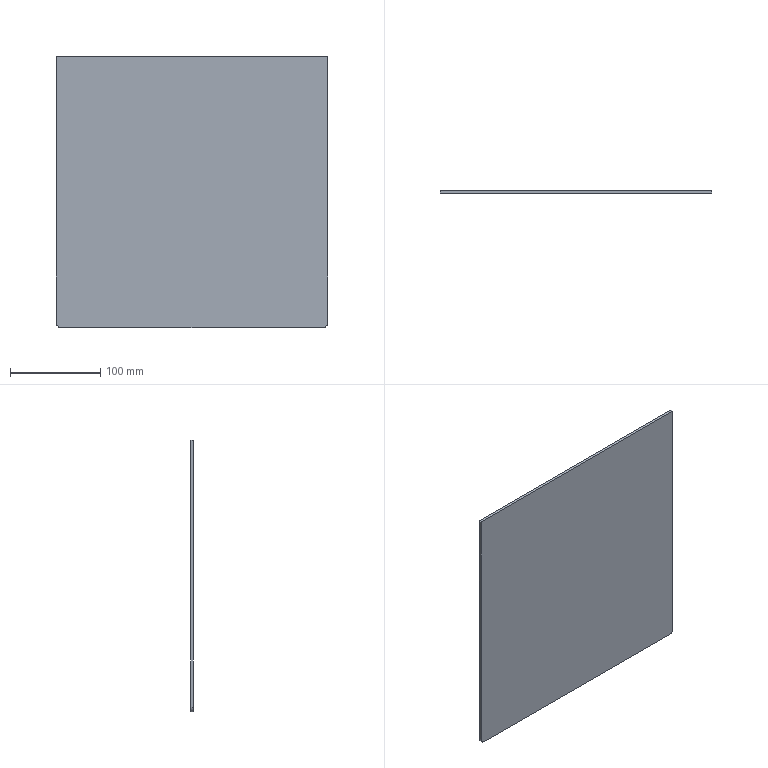Part | SolidWorks | features Extrusion 1 | 1 solid | 8 faces | box 300 x 3 x 300 mm | volume 269968 mm3 | plane 6 | cylinder 2 | commonest cylinder face diameters 10 x2
STEP:
#1=CARTESIAN_POINT('',(-150.,0.,-145.));
#2=VERTEX_POINT('',#1);
#3=CARTESIAN_POINT('',(-150.,0.,150.));
#4=VERTEX_POINT('',#3);
#5=CARTESIAN_POINT('',(-150.,0.,150.));
#6=DIRECTION('',(0.,0.,1.));
#7=VECTOR('',#6,1000.);
#8=LINE('',#5,#7);
#9=EDGE_CURVE('',#2,#4,#8,.T.);
#10=ORIENTED_EDGE('',*,*,#9,.T.);
#11=CARTESIAN_POINT('',(-150.,3.,150.));
#12=VERTEX_POINT('',#11);
#13=CARTESIAN_POINT('',(-150.,3.,150.));
#14=DIRECTION('',(0.,-1.,0.));
#15=VECTOR('',#14,1000.);
#16=LINE('',#13,#15);
#17=EDGE_CURVE('',#12,#4,#16,.T.);
#18=ORIENTED_EDGE('',*,*,#17,.F.);
#19=CARTESIAN_POINT('',(-150.,3.,-145.));
#20=VERTEX_POINT('',#19);
#21=CARTESIAN_POINT('',(-150.,3.,150.));
#22=DIRECTION('',(0.,0.,1.));
#23=VECTOR('',#22,1000.);
#24=LINE('',#21,#23);
#25=EDGE_CURVE('',#20,#12,#24,.T.);
#26=ORIENTED_EDGE('',*,*,#25,.F.);
#27=CARTESIAN_POINT('',(-150.,3.,-145.));
#28=DIRECTION('',(0.,-1.,0.));
#29=VECTOR('',#28,1000.);
#30=LINE('',#27,#29);
#31=EDGE_CURVE('',#20,#2,#30,.T.);
#32=ORIENTED_EDGE('',*,*,#31,.T.);
#33=EDGE_LOOP('',(#10,#18,#26,#32));
#34=FACE_OUTER_BOUND('',#33,.T.);
#35=CARTESIAN_POINT('',(-150.,3.,150.));
#36=DIRECTION('',(1.,0.,0.));
#37=DIRECTION('',(0.,0.,-1.));
#38=AXIS2_PLACEMENT_3D('',#35,#36,#37);
#39=PLANE('',#38);
#40=ADVANCED_FACE('',(#34),#39,.F.);
#41=CARTESIAN_POINT('',(150.,0.,150.));
#42=VERTEX_POINT('',#41);
#43=CARTESIAN_POINT('',(-150.,0.,150.));
#44=DIRECTION('',(1.,0.,0.));
#45=VECTOR('',#44,1000.);
#46=LINE('',#43,#45);
#47=EDGE_CURVE('',#4,#42,#46,.T.);
#48=ORIENTED_EDGE('',*,*,#47,.T.);
#49=CARTESIAN_POINT('',(150.,3.,150.));
#50=VERTEX_POINT('',#49);
#51=CARTESIAN_POINT('',(150.,3.,150.));
#52=DIRECTION('',(0.,-1.,0.));
#53=VECTOR('',#52,1000.);
#54=LINE('',#51,#53);
#55=EDGE_CURVE('',#50,#42,#54,.T.);
#56=ORIENTED_EDGE('',*,*,#55,.F.);
#57=CARTESIAN_POINT('',(-150.,3.,150.));
#58=DIRECTION('',(1.,0.,0.));
#59=VECTOR('',#58,1000.);
#60=LINE('',#57,#59);
#61=EDGE_CURVE('',#12,#50,#60,.T.);
#62=ORIENTED_EDGE('',*,*,#61,.F.);
#63=ORIENTED_EDGE('',*,*,#17,.T.);
#64=EDGE_LOOP('',(#48,#56,#62,#63));
#65=FACE_OUTER_BOUND('',#64,.T.);
#66=CARTESIAN_POINT('',(-150.,3.,150.));
#67=DIRECTION('',(0.,0.,-1.));
#68=DIRECTION('',(-1.,0.,0.));
#69=AXIS2_PLACEMENT_3D('',#66,#67,#68);
#70=PLANE('',#69);
#71=ADVANCED_FACE('',(#65),#70,.F.);
#72=CARTESIAN_POINT('',(150.,0.,-145.));
#73=VERTEX_POINT('',#72);
#74=CARTESIAN_POINT('',(150.,0.,150.));
#75=DIRECTION('',(0.,0.,-1.));
#76=VECTOR('',#75,1000.);
#77=LINE('',#74,#76);
#78=EDGE_CURVE('',#42,#73,#77,.T.);
#79=ORIENTED_EDGE('',*,*,#78,.T.);
#80=CARTESIAN_POINT('',(150.,3.,-145.));
#81=VERTEX_POINT('',#80);
#82=CARTESIAN_POINT('',(150.,3.,-145.));
#83=DIRECTION('',(0.,-1.,0.));
#84=VECTOR('',#83,1000.);
#85=LINE('',#82,#84);
#86=EDGE_CURVE('',#81,#73,#85,.T.);
#87=ORIENTED_EDGE('',*,*,#86,.F.);
#88=CARTESIAN_POINT('',(150.,3.,150.));
#89=DIRECTION('',(0.,0.,-1.));
#90=VECTOR('',#89,1000.);
#91=LINE('',#88,#90);
#92=EDGE_CURVE('',#50,#81,#91,.T.);
#93=ORIENTED_EDGE('',*,*,#92,.F.);
#94=ORIENTED_EDGE('',*,*,#55,.T.);
#95=EDGE_LOOP('',(#79,#87,#93,#94));
#96=FACE_OUTER_BOUND('',#95,.T.);
#97=CARTESIAN_POINT('',(150.,3.,150.));
#98=DIRECTION('',(-1.,0.,0.));
#99=DIRECTION('',(0.,0.,1.));
#100=AXIS2_PLACEMENT_3D('',#97,#98,#99);
#101=PLANE('',#100);
#102=ADVANCED_FACE('',(#96),#101,.F.);
#103=CARTESIAN_POINT('',(145.,0.,-150.));
#104=VERTEX_POINT('',#103);
#105=CARTESIAN_POINT('',(145.,0.,-145.));
#106=DIRECTION('',(0.,1.,0.));
#107=DIRECTION('',(0.,0.,-1.));
#108=AXIS2_PLACEMENT_3D('',#105,#106,#107);
#109=CIRCLE('',#108,5.);
#110=EDGE_CURVE('',#73,#104,#109,.T.);
#111=ORIENTED_EDGE('',*,*,#110,.T.);
#112=CARTESIAN_POINT('',(145.,3.,-150.));
#113=VERTEX_POINT('',#112);
#114=CARTESIAN_POINT('',(145.,3.,-150.));
#115=DIRECTION('',(0.,-1.,0.));
#116=VECTOR('',#115,1000.);
#117=LINE('',#114,#116);
#118=EDGE_CURVE('',#113,#104,#117,.T.);
#119=ORIENTED_EDGE('',*,*,#118,.F.);
#120=CARTESIAN_POINT('',(145.,3.,-145.));
#121=DIRECTION('',(0.,1.,0.));
#122=DIRECTION('',(0.,0.,-1.));
#123=AXIS2_PLACEMENT_3D('',#120,#121,#122);
#124=CIRCLE('',#123,5.);
#125=EDGE_CURVE('',#81,#113,#124,.T.);
#126=ORIENTED_EDGE('',*,*,#125,.F.);
#127=ORIENTED_EDGE('',*,*,#86,.T.);
#128=EDGE_LOOP('',(#111,#119,#126,#127));
#129=FACE_OUTER_BOUND('',#128,.T.);
#130=CARTESIAN_POINT('',(145.,3.,-145.));
#131=DIRECTION('',(0.,-1.,0.));
#132=DIRECTION('',(0.,0.,-1.));
#133=AXIS2_PLACEMENT_3D('',#130,#131,#132);
#134=CYLINDRICAL_SURFACE('',#133,5.);
#135=ADVANCED_FACE('',(#129),#134,.T.);
#136=CARTESIAN_POINT('',(-145.,0.,-150.));
#137=VERTEX_POINT('',#136);
#138=CARTESIAN_POINT('',(-145.,0.,-150.));
#139=DIRECTION('',(-1.,0.,0.));
#140=VECTOR('',#139,1000.);
#141=LINE('',#138,#140);
#142=EDGE_CURVE('',#104,#137,#141,.T.);
#143=ORIENTED_EDGE('',*,*,#142,.T.);
#144=CARTESIAN_POINT('',(-145.,3.,-150.));
#145=VERTEX_POINT('',#144);
#146=CARTESIAN_POINT('',(-145.,3.,-150.));
#147=DIRECTION('',(0.,-1.,0.));
#148=VECTOR('',#147,1000.);
#149=LINE('',#146,#148);
#150=EDGE_CURVE('',#145,#137,#149,.T.);
#151=ORIENTED_EDGE('',*,*,#150,.F.);
#152=CARTESIAN_POINT('',(-145.,3.,-150.));
#153=DIRECTION('',(-1.,0.,0.));
#154=VECTOR('',#153,1000.);
#155=LINE('',#152,#154);
#156=EDGE_CURVE('',#113,#145,#155,.T.);
#157=ORIENTED_EDGE('',*,*,#156,.F.);
#158=ORIENTED_EDGE('',*,*,#118,.T.);
#159=EDGE_LOOP('',(#143,#151,#157,#158));
#160=FACE_OUTER_BOUND('',#159,.T.);
#161=CARTESIAN_POINT('',(-145.,3.,-150.));
#162=DIRECTION('',(0.,0.,1.));
#163=DIRECTION('',(1.,0.,0.));
#164=AXIS2_PLACEMENT_3D('',#161,#162,#163);
#165=PLANE('',#164);
#166=ADVANCED_FACE('',(#160),#165,.F.);
#167=CARTESIAN_POINT('',(-145.,0.,-145.));
#168=DIRECTION('',(0.,1.,0.));
#169=DIRECTION('',(0.,0.,-1.));
#170=AXIS2_PLACEMENT_3D('',#167,#168,#169);
#171=CIRCLE('',#170,5.);
#172=EDGE_CURVE('',#137,#2,#171,.T.);
#173=ORIENTED_EDGE('',*,*,#172,.T.);
#174=ORIENTED_EDGE('',*,*,#31,.F.);
#175=CARTESIAN_POINT('',(-145.,3.,-145.));
#176=DIRECTION('',(0.,1.,0.));
#177=DIRECTION('',(0.,0.,-1.));
#178=AXIS2_PLACEMENT_3D('',#175,#176,#177);
#179=CIRCLE('',#178,5.);
#180=EDGE_CURVE('',#145,#20,#179,.T.);
#181=ORIENTED_EDGE('',*,*,#180,.F.);
#182=ORIENTED_EDGE('',*,*,#150,.T.);
#183=EDGE_LOOP('',(#173,#174,#181,#182));
#184=FACE_OUTER_BOUND('',#183,.T.);
#185=CARTESIAN_POINT('',(-145.,3.,-145.));
#186=DIRECTION('',(0.,-1.,0.));
#187=DIRECTION('',(0.,0.,-1.));
#188=AXIS2_PLACEMENT_3D('',#185,#186,#187);
#189=CYLINDRICAL_SURFACE('',#188,5.);
#190=ADVANCED_FACE('',(#184),#189,.T.);
#191=ORIENTED_EDGE('',*,*,#25,.T.);
#192=ORIENTED_EDGE('',*,*,#61,.T.);
#193=ORIENTED_EDGE('',*,*,#92,.T.);
#194=ORIENTED_EDGE('',*,*,#125,.T.);
#195=ORIENTED_EDGE('',*,*,#156,.T.);
#196=ORIENTED_EDGE('',*,*,#180,.T.);
#197=EDGE_LOOP('',(#191,#192,#193,#194,#195,#196));
#198=FACE_OUTER_BOUND('',#197,.T.);
#199=CARTESIAN_POINT('',(-145.,3.,-145.));
#200=DIRECTION('',(0.,-1.,0.));
#201=DIRECTION('',(0.,0.,-1.));
#202=AXIS2_PLACEMENT_3D('',#199,#200,#201);
#203=PLANE('',#202);
#204=ADVANCED_FACE('',(#198),#203,.F.);
#205=ORIENTED_EDGE('',*,*,#9,.F.);
#206=ORIENTED_EDGE('',*,*,#172,.F.);
#207=ORIENTED_EDGE('',*,*,#142,.F.);
#208=ORIENTED_EDGE('',*,*,#110,.F.);
#209=ORIENTED_EDGE('',*,*,#78,.F.);
#210=ORIENTED_EDGE('',*,*,#47,.F.);
#211=EDGE_LOOP('',(#205,#206,#207,#208,#209,#210));
#212=FACE_OUTER_BOUND('',#211,.T.);
#213=CARTESIAN_POINT('',(-145.,0.,-145.));
#214=DIRECTION('',(0.,-1.,0.));
#215=DIRECTION('',(0.,0.,-1.));
#216=AXIS2_PLACEMENT_3D('',#213,#214,#215);
#217=PLANE('',#216);
#218=ADVANCED_FACE('',(#212),#217,.T.);
#219=CLOSED_SHELL('',(#40,#71,#102,#135,#166,#190,#204,#218));
#220=MANIFOLD_SOLID_BREP('',#219);
#221=CARTESIAN_POINT('',(0.,0.,0.));
#222=DIRECTION('',(0.,0.,1.));
#223=DIRECTION('',(1.,0.,0.));
#224=AXIS2_PLACEMENT_3D('',#221,#222,#223);
#225=(LENGTH_UNIT()NAMED_UNIT(*)SI_UNIT(.MILLI.,.METRE.));
#226=UNCERTAINTY_MEASURE_WITH_UNIT(LENGTH_MEASURE(0.00001),#225,'','');
#227=(NAMED_UNIT(*)PLANE_ANGLE_UNIT()SI_UNIT($,.RADIAN.));
#228=(NAMED_UNIT(*)SI_UNIT($,.STERADIAN.)SOLID_ANGLE_UNIT());
#229=(GEOMETRIC_REPRESENTATION_CONTEXT(3)GLOBAL_UNCERTAINTY_ASSIGNED_CONTEXT((#226))GLOBAL_UNIT_ASSIGNED_CONTEXT((#225,#227,#228))REPRESENTATION_CONTEXT('',''));
#230=ADVANCED_BREP_SHAPE_REPRESENTATION('',(#220,#224),#229);